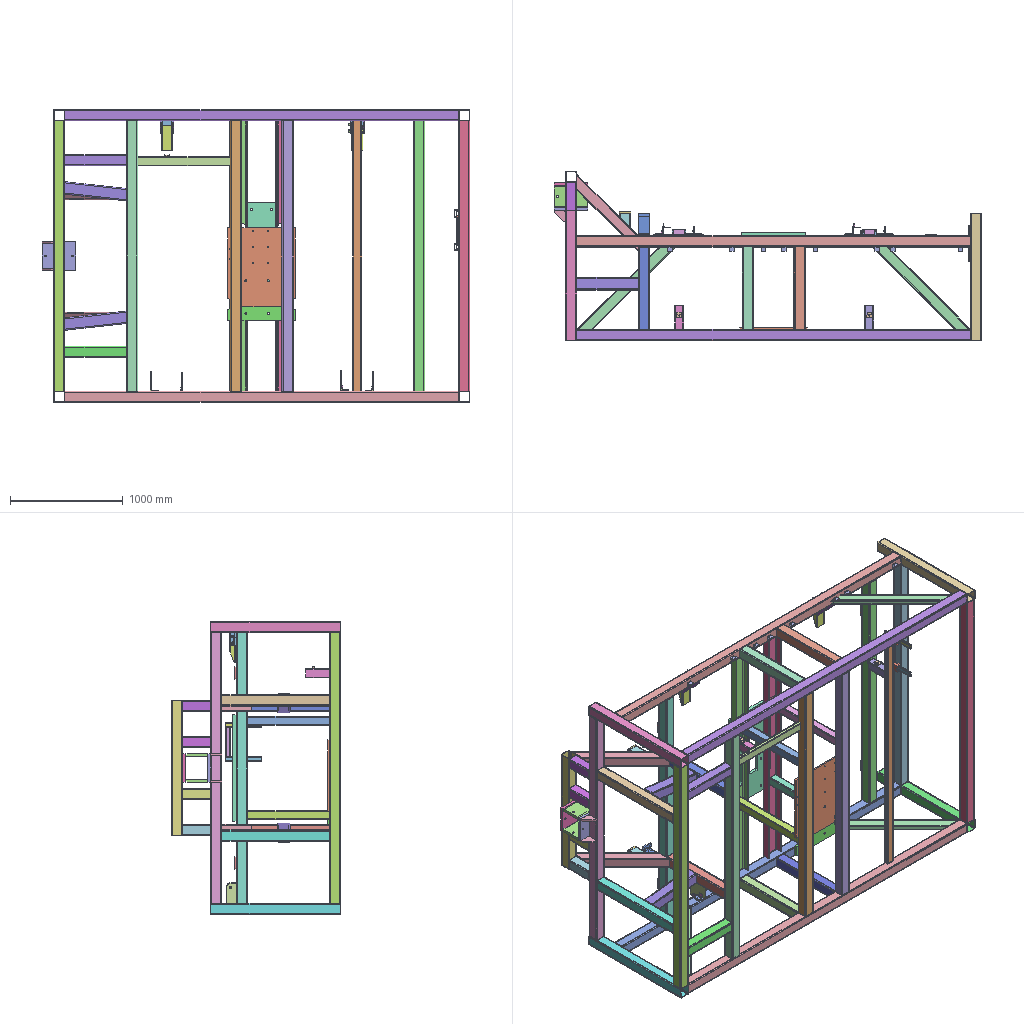Assembly | SolidWorks | 25 different items | 67 placed | box 3800 x 1505 x 2600 mm
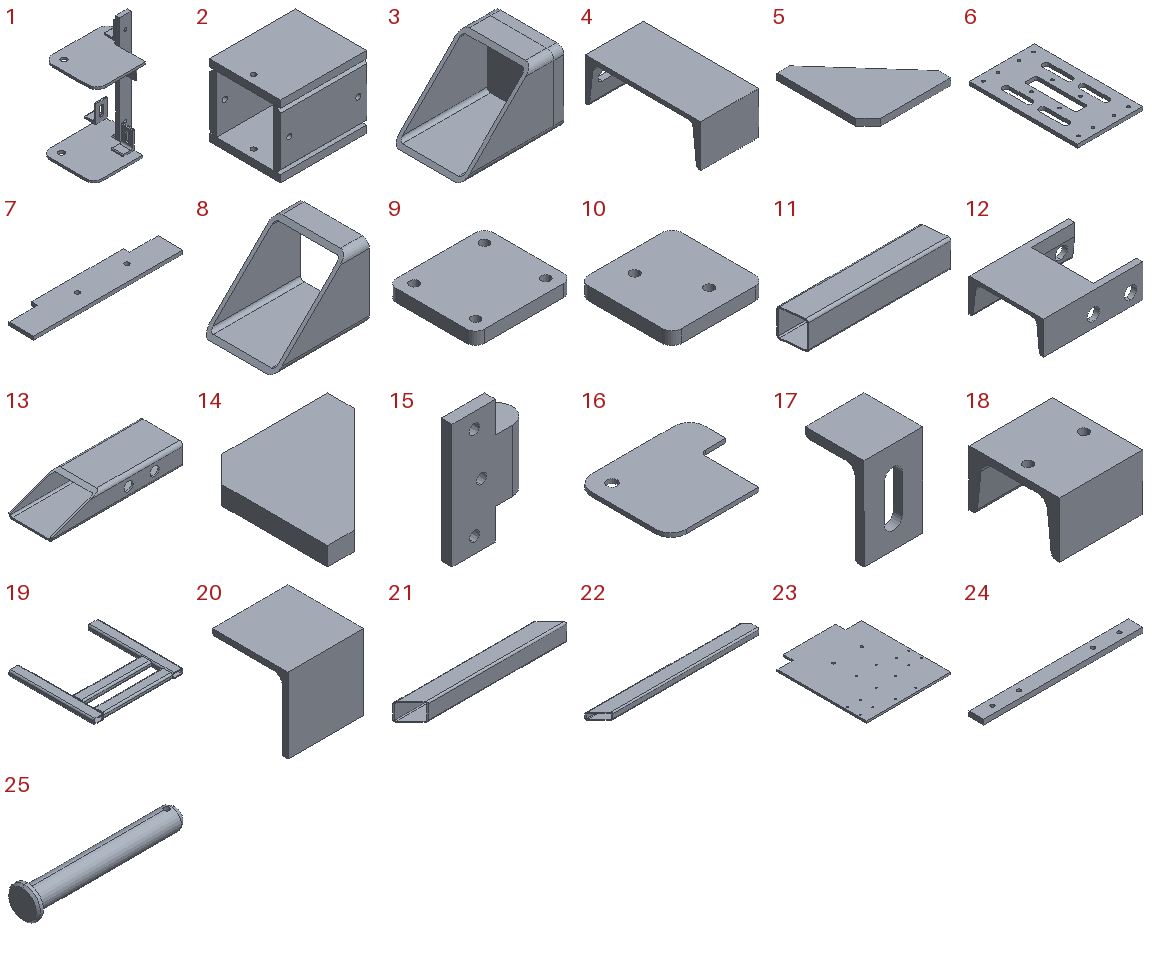Parts list (item | name | quantity | parent item | size | volume | features):
1 | (subassembly) | x2 | - | 228.637 x 214.539 x 440 mm | 910325 mm3 | -
2 | (subassembly) | x1 | - | 300 x 250 x 250 mm | 6572908 mm3 | -
3 | (subassembly) | x1 | - | 144 x 100 x 100 mm | 283360 mm3 | -
4 | - | x2 | - | 100 x 200 x 73 mm | 272858 mm3 | features 3DProfileFeature 1, ICE 1, WeldMemberFeat 1, WeldmentFeature 1
5 | - | x4 | - | 100 x 110 x 8 mm | 54800 mm3 | features Chamfer 1, Extrusion 1
6 | - | x1 | - | 570 x 950 x 30 mm | 12981435 mm3 | features Extrusion 1
7 | - | x1 | - | 600 x 125 x 14 mm | 962375 mm3 | features Extrusion 1
8 | - | x2 | in 3 | 130 x 100 x 100 mm | 146850 mm3 | features 3DProfileFeature 1, Cut 1, WeldMemberFeat 1, WeldmentFeature 1
9 | - | x4 | - | 110 x 100 x 14 mm | 148222 mm3 | features 3DProfileFeature 1, Extrusion 1, HoleWzd 1
10 | - | x2 | in 3 | 100 x 100 x 14 mm | 136510 mm3 | features 3DProfileFeature 1, Extrusion 1, Fillet 1, HoleWzd 1
11 | - | x2 | - | 565.469 x 110 x 110 mm | 1126381 mm3 | features 3DProfileFeature 1, ICE 1, WeldMemberFeat 1, WeldmentFeature 1
12 | - | x2 | - | 160 x 120 x 53 mm | 192954 mm3 | features ICE 2, 3DProfileFeature 1, WeldMemberFeat 1, WeldmentFeature 1
13 | - | x2 | - | 300 x 100 x 50 mm | 365371 mm3 | features ICE 2, 3DProfileFeature 1, WeldMemberFeat 1, WeldmentFeature 1
14 | - | x2 | - | 100 x 100 x 14 mm | 92400 mm3 | features Extrusion 1
15 | - | x2 | - | 49.5 x 21 x 80 mm | 29616 mm3 | features BaseBody 1
16 | - | x4 | in 1 | 220 x 184 x 8 mm | 271263 mm3 | features Extrusion 1
17 | - | x12 | in 1 | 40 x 40 x 63 mm | 20996 mm3 | features 3DProfileFeature 1, Cut 1, WeldMemberFeat 1, WeldmentFeature 1
18 | - | x2 | - | 60 x 65 x 40 mm | 50891 mm3 | features 3DProfileFeature 2, HoleWzd 1, WeldMemberFeat 1, WeldmentFeature 1
19 | - | x1 | - | 340 x 320 x 20 mm | 348955 mm3 | features 3DProfileFeature 1, WeldMemberFeat 1, WeldmentFeature 1
20 | - | x8 | - | 40 x 40 x 40 mm | 9437 mm3 | features 3DProfileFeature 1, WeldMemberFeat 1, WeldmentFeature 1
21 | - | x2 | - | 877.817 x 100 x 100 mm | 1427777 mm3 | features 3DProfileFeature 1, ICE 1, WeldMemberFeat 1, WeldmentFeature 1
22 | - | x3 | - | 1150 x 100 x 50 mm | 1450774 mm3 | features 3DProfileFeature 1, ICE 1, WeldMemberFeat 1, WeldmentFeature 1
23 | - | x1 | - | 600 x 700 x 14 mm | 5631459 mm3 | features 3DProfileFeature 1, Extrusion 1, HoleWzd 1
24 | - | x2 | in 1 | 440 x 40 x 14 mm | 241824 mm3 | features 3DProfileFeature 1, Extrusion 1, HoleWzd 1
25 | - | x2 | - | 145 x 30 x 30 mm | 46693 mm3 | features Chamfer 1, Fillet 1, ICE 1, Revolution 1
Mates (type | each side: item.copy, entity, surface, feature):
In the top assembly
Concentric | 12.1 face cylinder Cut-Extrude2 | 13.1 face cylinder Cut-Extrude1 | 2 times
DistanceDim | 13.1 face plane Rectangular tube 100 X 50 X 4(1) | 12.1 face plane C Channel 12(1)
Coincident | 21.1 face plane Square tube 100 X 100 X 5(1) | 8.1 face plane Square tube 100 X 100 X 5   (1)
Coincident | 8.1 face plane Square tube 100 X 100 X 5   (1) | 8.2 face plane Square tube 100 X 100 X 5   (1)
Coincident | 21.2 face plane Square tube 100 X 100 X 5(1) | 8.2 face plane Square tube 100 X 100 X 5   (1)
Coincident | 10.1 face plane Boss-Extrude1 | 8.2 face plane Square tube 100 X 100 X 5   (1) | 3 times
Coincident | 12.1 face plane C Channel 12(1) | 5.1 face plane Boss-Extrude1 | 2 times
Coincident | 12.1 face plane C Channel 12(1) | 5.2 face plane Boss-Extrude1 | 2 times
Concentric | 12.2 face cylinder Cut-Extrude2 | 13.2 face cylinder Cut-Extrude1 | 2 times
DistanceDim | 13.2 face plane Rectangular tube 100 X 50 X 4(1) | 12.2 face plane C Channel 12(1)
Coincident | 12.2 face plane C Channel 12(1) | 5.3 face plane Boss-Extrude1 | 2 times
Coincident | 12.2 face plane C Channel 12(1) | 5.4 face plane Boss-Extrude1 | 2 times
Coincident | 9.1 face plane Boss-Extrude1 | 9.2 face plane Boss-Extrude1
Coincident | 9.3 face plane Boss-Extrude1 | 9.4 face plane Boss-Extrude1
Coincident | 4.1 face plane C Channel 20A(1) | 4.2 face plane C Channel 20A(1)
Coincident | 11.1 face plane Square tube 110 X 110 X 5(1) | 11.2 face plane Square tube 110 X 110 X 5(1)
Coincident | 21.1 face plane Square tube 100 X 100 X 5(1) | 8.1 face plane Cut-Extrude1
Coincident | 21.2 face plane Square tube 100 X 100 X 5(1) | 8.2 face plane Cut-Extrude1
Coincident | 23.1 face plane Boss-Extrude1 | 7.1 face plane Boss-Extrude1 | 2 times
Coincident | 19.1 face plane Rectangular tube 40 X 20 X 3(1) | 18.1 face plane C Channel 6.5(1)
DistanceDim | 18.1 face plane C Channel 6.5(1) | 19.1 face plane Rectangular tube 40 X 20 X 3(1)
Coincident | 18.1 face plane C Channel 6.5(1) | 18.2 face plane C Channel 6.5(1) | 2 times
DistanceDim | 19.1 face plane Rectangular tube 40 X 20 X 3(1) | 18.2 face plane C Channel 6.5(1)
Coincident | 20.1 face plane Angle iron 40 X 3(1) | 20.2 face plane Angle iron 40 X 3(1)
DistanceDim | 20.2 face plane Angle iron 40 X 3(1) | 20.1 face plane Angle iron 40 X 3(1)
Coincident | 20.3 face plane Angle iron 40 X 3(1) | 20.4 face plane Angle iron 40 X 3(1)
Coincident | 20.3 face plane Angle iron 40 X 3(1) | 20.5 face plane Angle iron 40 X 3(1)
Coincident | 20.5 face plane Angle iron 40 X 3(1) | 20.6 face plane Angle iron 40 X 3(1)
Coincident | 20.5 face plane Angle iron 40 X 3(1) | 20.7 face plane Angle iron 40 X 3(1)
DistanceDim | 20.5 face plane Angle iron 40 X 3(1) | 20.7 face plane Angle iron 40 X 3(1)
Coincident | 20.7 face plane Angle iron 40 X 3(1) | 20.8 face plane Angle iron 40 X 3(1)
DistanceDim | 20.8 face plane Angle iron 40 X 3(1) | 20.6 face plane Angle iron 40 X 3(1)
Concentric | 12.1 face cylinder Cut-Extrude2 | 25.1 face cylinder Base-Revolve
Coincident | 12.1 face plane C Channel 12(1) | 25.1 face plane Base-Revolve
Concentric | 12.1 face cylinder Cut-Extrude2 | 25.2 face cylinder Base-Revolve
Coincident | 12.1 face plane C Channel 12(1) | 25.2 face plane Base-Revolve
Parallel | 12.1 face plane C Channel 12(1) | 25.2 axis
Parallel | 12.1 face plane C Channel 12(1) | 25.1 axis
In subassembly 3
InPlace | 8.2 face plane Square tube 100 X 100 X 5   (1) | 10.1 plane
In subassembly 1
Coincident | 16.1 face plane Boss-Extrude1 | 17.1 face plane Hot-rolled unequal angle steel gb∕t706-2008 63 X 40 X 6(1)
Coincident | 17.2 face plane Hot-rolled unequal angle steel gb∕t706-2008 63 X 40 X 6(1) | 17.1 face plane Hot-rolled unequal angle steel gb∕t706-2008 63 X 40 X 6(1) | 2 times
Coincident | 17.2 face plane Hot-rolled unequal angle steel gb∕t706-2008 63 X 40 X 6(1) | 24.1 face plane Boss-Extrude1 | 2 times
DistanceDim | 24.1 axis | 17.1 axis
Coincident | 16.2 face plane Boss-Extrude1 | 17.3 face plane Hot-rolled unequal angle steel gb∕t706-2008 63 X 40 X 6(1) | 3 times
Coincident | 24.1 face plane Boss-Extrude1 | 16.2 face plane Boss-Extrude1
Coincident | 16.2 face plane Boss-Extrude1 | 17.4 face plane Hot-rolled unequal angle steel gb∕t706-2008 63 X 40 X 6(1)
Coincident | 24.1 face plane Boss-Extrude1 | 17.4 face plane Hot-rolled unequal angle steel gb∕t706-2008 63 X 40 X 6(1)
Coincident | 17.3 face plane Hot-rolled unequal angle steel gb∕t706-2008 63 X 40 X 6(1) | 17.4 face plane Hot-rolled unequal angle steel gb∕t706-2008 63 X 40 X 6(1)
DistanceDim | 16.2 face plane Boss-Extrude1 | 16.1 face plane Boss-Extrude1
Coincident | 16.1 face plane Boss-Extrude1 | 17.5 face plane Hot-rolled unequal angle steel gb∕t706-2008 63 X 40 X 6(1) | 2 times
DistanceDim | 17.5 face plane Hot-rolled unequal angle steel gb∕t706-2008 63 X 40 X 6(1) | 16.1 face plane Boss-Extrude1
Coincident | 16.2 face plane Boss-Extrude1 | 17.6 face plane Hot-rolled unequal angle steel gb∕t706-2008 63 X 40 X 6(1) | 2 times
Coincident | 17.5 face plane Hot-rolled unequal angle steel gb∕t706-2008 63 X 40 X 6(1) | 17.6 face plane Hot-rolled unequal angle steel gb∕t706-2008 63 X 40 X 6(1)